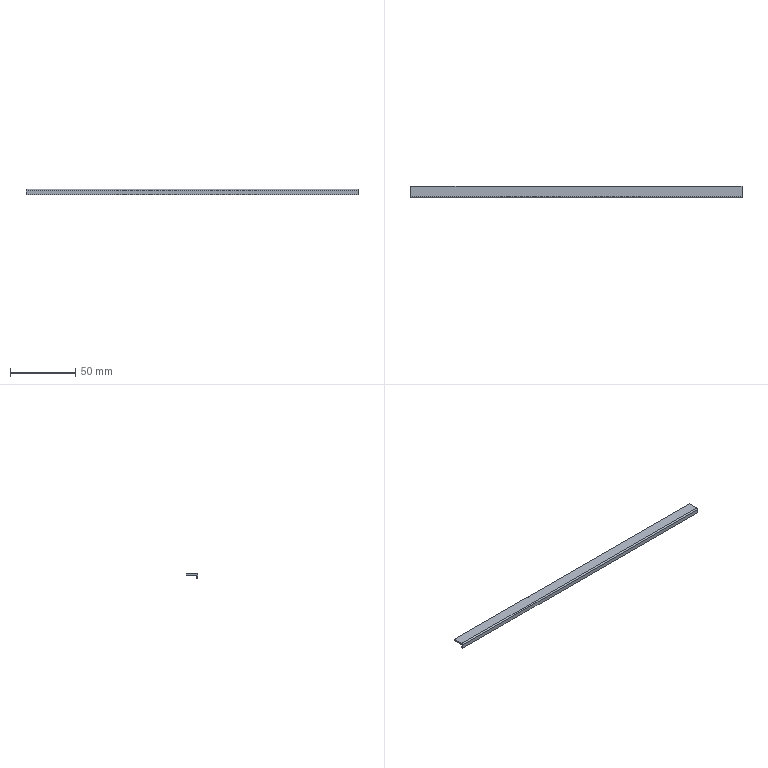Part | STEP file | gslz 2016.10.28-13_id966_x_t | 1 solid | 12 faces | box 255.209 x 9 x 4 mm | volume 3693 mm3 | plane 9 | cylinder 3 | commonest cylinder face diameters 4 x2 2 x1
STEP:
#1=CARTESIAN_POINT('',(0.,0.,0.));
#2=DIRECTION('',(0.,0.,1.));
#3=DIRECTION('',(1.,0.,0.));
#4=AXIS2_PLACEMENT_3D('',#1,#2,#3);
#5=CARTESIAN_POINT('',(-377.345,-257.,0.));
#6=VERTEX_POINT('',#5);
#7=CARTESIAN_POINT('',(-551.382,-257.,0.));
#8=VERTEX_POINT('',#7);
#9=CARTESIAN_POINT('',(-428.432,-257.,0.));
#10=DIRECTION('',(-1.,0.,0.));
#11=VECTOR('',#10,1.);
#12=LINE('',#9,#11);
#13=CARTESIAN_POINT('',(-428.432,-257.,2.5));
#14=DIRECTION('',(0.,-1.,0.));
#15=DIRECTION('',(1.,0.,0.));
#16=AXIS2_PLACEMENT_3D('',#13,#14,#15);
#17=PLANE('',#16);
#18=CARTESIAN_POINT('',(0.,-2.5));
#19=DIRECTION('',(-1.,0.));
#20=VECTOR('',#19,1.);
#21=LINE('',#18,#20);
#22=(GEOMETRIC_REPRESENTATION_CONTEXT(2)PARAMETRIC_REPRESENTATION_CONTEXT()REPRESENTATION_CONTEXT('',''));
#23=DEFINITIONAL_REPRESENTATION('',(#21),#22);
#24=PCURVE('',#17,#23);
#25=CARTESIAN_POINT('',(1793.591,319.067,0.));
#26=DIRECTION('',(0.,0.,1.));
#27=DIRECTION('',(1.,0.,0.));
#28=AXIS2_PLACEMENT_3D('',#25,#26,#27);
#29=PLANE('',#28);
#30=CARTESIAN_POINT('',(-2222.023,-576.067));
#31=DIRECTION('',(-1.,0.));
#32=VECTOR('',#31,1.);
#33=LINE('',#30,#32);
#34=(GEOMETRIC_REPRESENTATION_CONTEXT(2)PARAMETRIC_REPRESENTATION_CONTEXT()REPRESENTATION_CONTEXT('',''));
#35=DEFINITIONAL_REPRESENTATION('',(#33),#34);
#36=PCURVE('',#29,#35);
#37=SURFACE_CURVE('',#12,(#24,#36),.PCURVE_S1.);
#38=EDGE_CURVE('',#6,#8,#37,.T.);
#39=ORIENTED_EDGE('',*,*,#38,.T.);
#40=CARTESIAN_POINT('',(-551.382,-257.,1.25));
#41=VERTEX_POINT('',#40);
#42=CARTESIAN_POINT('',(-551.382,-257.,2.5));
#43=DIRECTION('',(0.,0.,-1.));
#44=VECTOR('',#43,1.);
#45=LINE('',#42,#44);
#46=CARTESIAN_POINT('',(-122.95,0.));
#47=DIRECTION('',(0.,-1.));
#48=VECTOR('',#47,1.);
#49=LINE('',#46,#48);
#50=(GEOMETRIC_REPRESENTATION_CONTEXT(2)PARAMETRIC_REPRESENTATION_CONTEXT()REPRESENTATION_CONTEXT('',''));
#51=DEFINITIONAL_REPRESENTATION('',(#49),#50);
#52=PCURVE('',#17,#51);
#53=CARTESIAN_POINT('',(-552.435,-255.3,2.5));
#54=DIRECTION('',(0.,0.,-1.));
#55=DIRECTION('',(-1.,0.,0.));
#56=AXIS2_PLACEMENT_3D('',#53,#54,#55);
#57=CYLINDRICAL_SURFACE('',#56,2.);
#58=CARTESIAN_POINT('',(4.158,0.));
#59=DIRECTION('',(0.,1.));
#60=VECTOR('',#59,1.);
#61=LINE('',#58,#60);
#62=(GEOMETRIC_REPRESENTATION_CONTEXT(2)PARAMETRIC_REPRESENTATION_CONTEXT()REPRESENTATION_CONTEXT('',''));
#63=DEFINITIONAL_REPRESENTATION('',(#61),#62);
#64=PCURVE('',#57,#63);
#65=SURFACE_CURVE('',#45,(#52,#64),.PCURVE_S1.);
#66=EDGE_CURVE('',#41,#8,#65,.T.);
#67=ORIENTED_EDGE('',*,*,#66,.F.);
#68=CARTESIAN_POINT('',(-377.345,-257.,1.25));
#69=VERTEX_POINT('',#68);
#70=CARTESIAN_POINT('',(1793.591,-257.,1.25));
#71=DIRECTION('',(1.,0.,0.));
#72=VECTOR('',#71,1.);
#73=LINE('',#70,#72);
#74=CARTESIAN_POINT('',(2222.023,-1.25));
#75=DIRECTION('',(1.,0.));
#76=VECTOR('',#75,1.);
#77=LINE('',#74,#76);
#78=(GEOMETRIC_REPRESENTATION_CONTEXT(2)PARAMETRIC_REPRESENTATION_CONTEXT()REPRESENTATION_CONTEXT('',''));
#79=DEFINITIONAL_REPRESENTATION('',(#77),#78);
#80=PCURVE('',#17,#79);
#81=CARTESIAN_POINT('',(1793.591,319.067,1.25));
#82=DIRECTION('',(0.,0.,1.));
#83=DIRECTION('',(1.,0.,0.));
#84=AXIS2_PLACEMENT_3D('',#81,#82,#83);
#85=PLANE('',#84);
#86=CARTESIAN_POINT('',(0.,-576.067));
#87=DIRECTION('',(1.,0.));
#88=VECTOR('',#87,1.);
#89=LINE('',#86,#88);
#90=(GEOMETRIC_REPRESENTATION_CONTEXT(2)PARAMETRIC_REPRESENTATION_CONTEXT()REPRESENTATION_CONTEXT('',''));
#91=DEFINITIONAL_REPRESENTATION('',(#89),#90);
#92=PCURVE('',#85,#91);
#93=SURFACE_CURVE('',#73,(#80,#92),.PCURVE_S1.);
#94=EDGE_CURVE('',#41,#69,#93,.T.);
#95=ORIENTED_EDGE('',*,*,#94,.T.);
#96=CARTESIAN_POINT('',(-377.345,-257.,-0.75));
#97=DIRECTION('',(0.,0.,1.));
#98=VECTOR('',#97,1.);
#99=LINE('',#96,#98);
#100=CARTESIAN_POINT('',(51.087,-3.25));
#101=DIRECTION('',(0.,1.));
#102=VECTOR('',#101,1.);
#103=LINE('',#100,#102);
#104=(GEOMETRIC_REPRESENTATION_CONTEXT(2)PARAMETRIC_REPRESENTATION_CONTEXT()REPRESENTATION_CONTEXT('',''));
#105=DEFINITIONAL_REPRESENTATION('',(#103),#104);
#106=PCURVE('',#17,#105);
#107=CARTESIAN_POINT('',(-377.345,-275.25,-0.75));
#108=DIRECTION('',(-1.,0.,0.));
#109=DIRECTION('',(0.,-1.,0.));
#110=AXIS2_PLACEMENT_3D('',#107,#108,#109);
#111=PLANE('',#110);
#112=CARTESIAN_POINT('',(-18.25,0.));
#113=DIRECTION('',(0.,1.));
#114=VECTOR('',#113,1.);
#115=LINE('',#112,#114);
#116=(GEOMETRIC_REPRESENTATION_CONTEXT(2)PARAMETRIC_REPRESENTATION_CONTEXT()REPRESENTATION_CONTEXT('',''));
#117=DEFINITIONAL_REPRESENTATION('',(#115),#116);
#118=PCURVE('',#111,#117);
#119=SURFACE_CURVE('',#99,(#106,#118),.PCURVE_S1.);
#120=EDGE_CURVE('',#6,#69,#119,.T.);
#121=ORIENTED_EDGE('',*,*,#120,.F.);
#122=EDGE_LOOP('',(#39,#67,#95,#121));
#123=FACE_BOUND('',#122,.T.);
#124=ADVANCED_FACE('',(#123),#17,.F.);
#125=CARTESIAN_POINT('',(-553.195,-257.15,1.25));
#126=VERTEX_POINT('',#125);
#127=CARTESIAN_POINT('',(-552.435,-255.3,1.25));
#128=DIRECTION('',(0.,0.,-1.));
#129=DIRECTION('',(1.,0.,0.));
#130=AXIS2_PLACEMENT_3D('',#127,#128,#129);
#131=CIRCLE('',#130,2.);
#132=CARTESIAN_POINT('',(3.142,1.25));
#133=DIRECTION('',(1.,0.));
#134=VECTOR('',#133,1.);
#135=LINE('',#132,#134);
#136=(GEOMETRIC_REPRESENTATION_CONTEXT(2)PARAMETRIC_REPRESENTATION_CONTEXT()REPRESENTATION_CONTEXT('',''));
#137=DEFINITIONAL_REPRESENTATION('',(#135),#136);
#138=PCURVE('',#57,#137);
#139=CARTESIAN_POINT('',(-2344.027,-574.367));
#140=CARTESIAN_POINT('',(-2344.027,-577.831));
#141=CARTESIAN_POINT('',(-2347.027,-576.099));
#142=CARTESIAN_POINT('',(-2350.027,-574.367));
#143=CARTESIAN_POINT('',(-2347.027,-572.635));
#144=CARTESIAN_POINT('',(-2344.027,-570.903));
#145=CARTESIAN_POINT('',(-2344.027,-574.367));
#146=(BOUNDED_CURVE()B_SPLINE_CURVE(2,(#139,#140,#141,#142,#143,#144,#145),.UNSPECIFIED.,.T.,.F.)B_SPLINE_CURVE_WITH_KNOTS((1,2,2,2,2,1),(-2.094,0.,2.094,4.189,6.283,8.378),.UNSPECIFIED.)CURVE()GEOMETRIC_REPRESENTATION_ITEM()RATIONAL_B_SPLINE_CURVE((1.,0.5,1.,0.5,1.,0.5,1.))REPRESENTATION_ITEM(''));
#147=(GEOMETRIC_REPRESENTATION_CONTEXT(2)PARAMETRIC_REPRESENTATION_CONTEXT()REPRESENTATION_CONTEXT('',''));
#148=DEFINITIONAL_REPRESENTATION('',(#146),#147);
#149=PCURVE('',#85,#148);
#150=SURFACE_CURVE('',#131,(#138,#149),.PCURVE_S1.);
#151=EDGE_CURVE('',#41,#126,#150,.T.);
#152=ORIENTED_EDGE('',*,*,#151,.T.);
#153=CARTESIAN_POINT('',(-553.195,-257.15,0.));
#154=VERTEX_POINT('',#153);
#155=CARTESIAN_POINT('',(-553.195,-257.15,2.5));
#156=DIRECTION('',(0.,0.,1.));
#157=VECTOR('',#156,1.);
#158=LINE('',#155,#157);
#159=CARTESIAN_POINT('',(5.102,0.));
#160=DIRECTION('',(0.,-1.));
#161=VECTOR('',#160,1.);
#162=LINE('',#159,#161);
#163=(GEOMETRIC_REPRESENTATION_CONTEXT(2)PARAMETRIC_REPRESENTATION_CONTEXT()REPRESENTATION_CONTEXT('',''));
#164=DEFINITIONAL_REPRESENTATION('',(#162),#163);
#165=PCURVE('',#57,#164);
#166=CARTESIAN_POINT('',(-553.955,-259.,2.5));
#167=DIRECTION('',(0.,0.,-1.));
#168=DIRECTION('',(-1.,0.,0.));
#169=AXIS2_PLACEMENT_3D('',#166,#167,#168);
#170=CYLINDRICAL_SURFACE('',#169,2.);
#171=CARTESIAN_POINT('',(1.961,0.));
#172=DIRECTION('',(0.,-1.));
#173=VECTOR('',#172,1.);
#174=LINE('',#171,#173);
#175=(GEOMETRIC_REPRESENTATION_CONTEXT(2)PARAMETRIC_REPRESENTATION_CONTEXT()REPRESENTATION_CONTEXT('',''));
#176=DEFINITIONAL_REPRESENTATION('',(#174),#175);
#177=PCURVE('',#170,#176);
#178=SURFACE_CURVE('',#158,(#165,#177),.PCURVE_S1.);
#179=EDGE_CURVE('',#154,#126,#178,.T.);
#180=ORIENTED_EDGE('',*,*,#179,.F.);
#181=CARTESIAN_POINT('',(-552.435,-255.3,0.));
#182=DIRECTION('',(0.,0.,1.));
#183=DIRECTION('',(1.,0.,0.));
#184=AXIS2_PLACEMENT_3D('',#181,#182,#183);
#185=CIRCLE('',#184,2.);
#186=CARTESIAN_POINT('',(9.425,2.5));
#187=DIRECTION('',(-1.,0.));
#188=VECTOR('',#187,1.);
#189=LINE('',#186,#188);
#190=(GEOMETRIC_REPRESENTATION_CONTEXT(2)PARAMETRIC_REPRESENTATION_CONTEXT()REPRESENTATION_CONTEXT('',''));
#191=DEFINITIONAL_REPRESENTATION('',(#189),#190);
#192=PCURVE('',#57,#191);
#193=CARTESIAN_POINT('',(-2346.027,-574.367));
#194=DIRECTION('',(1.,0.));
#195=AXIS2_PLACEMENT_2D('',#193,#194);
#196=CIRCLE('',#195,2.);
#197=(GEOMETRIC_REPRESENTATION_CONTEXT(2)PARAMETRIC_REPRESENTATION_CONTEXT()REPRESENTATION_CONTEXT('',''));
#198=DEFINITIONAL_REPRESENTATION('',(#196),#197);
#199=PCURVE('',#29,#198);
#200=SURFACE_CURVE('',#185,(#192,#199),.PCURVE_S1.);
#201=EDGE_CURVE('',#154,#8,#200,.T.);
#202=ORIENTED_EDGE('',*,*,#201,.T.);
#203=ORIENTED_EDGE('',*,*,#66,.F.);
#204=EDGE_LOOP('',(#152,#180,#202,#203));
#205=FACE_BOUND('',#204,.F.);
#206=ADVANCED_FACE('',(#205),#57,.F.);
#207=ORIENTED_EDGE('',*,*,#179,.F.);
#208=CARTESIAN_POINT('',(-553.955,-257.,0.));
#209=VERTEX_POINT('',#208);
#210=CARTESIAN_POINT('',(-553.955,-259.,0.));
#211=DIRECTION('',(0.,0.,-1.));
#212=DIRECTION('',(1.,0.,0.));
#213=AXIS2_PLACEMENT_3D('',#210,#211,#212);
#214=CIRCLE('',#213,2.);
#215=CARTESIAN_POINT('',(-3.142,2.5));
#216=DIRECTION('',(1.,0.));
#217=VECTOR('',#216,1.);
#218=LINE('',#215,#217);
#219=(GEOMETRIC_REPRESENTATION_CONTEXT(2)PARAMETRIC_REPRESENTATION_CONTEXT()REPRESENTATION_CONTEXT('',''));
#220=DEFINITIONAL_REPRESENTATION('',(#218),#219);
#221=PCURVE('',#170,#220);
#222=CARTESIAN_POINT('',(-2345.546,-578.067));
#223=CARTESIAN_POINT('',(-2345.546,-581.531));
#224=CARTESIAN_POINT('',(-2348.546,-579.799));
#225=CARTESIAN_POINT('',(-2351.546,-578.067));
#226=CARTESIAN_POINT('',(-2348.546,-576.335));
#227=CARTESIAN_POINT('',(-2345.546,-574.603));
#228=CARTESIAN_POINT('',(-2345.546,-578.067));
#229=(BOUNDED_CURVE()B_SPLINE_CURVE(2,(#222,#223,#224,#225,#226,#227,#228),.UNSPECIFIED.,.T.,.F.)B_SPLINE_CURVE_WITH_KNOTS((1,2,2,2,2,1),(-2.094,0.,2.094,4.189,6.283,8.378),.UNSPECIFIED.)CURVE()GEOMETRIC_REPRESENTATION_ITEM()RATIONAL_B_SPLINE_CURVE((1.,0.5,1.,0.5,1.,0.5,1.))REPRESENTATION_ITEM(''));
#230=(GEOMETRIC_REPRESENTATION_CONTEXT(2)PARAMETRIC_REPRESENTATION_CONTEXT()REPRESENTATION_CONTEXT('',''));
#231=DEFINITIONAL_REPRESENTATION('',(#229),#230);
#232=PCURVE('',#29,#231);
#233=SURFACE_CURVE('',#214,(#221,#232),.PCURVE_S1.);
#234=EDGE_CURVE('',#209,#154,#233,.T.);
#235=ORIENTED_EDGE('',*,*,#234,.F.);
#236=CARTESIAN_POINT('',(-553.955,-257.,1.25));
#237=VERTEX_POINT('',#236);
#238=CARTESIAN_POINT('',(-553.955,-257.,2.5));
#239=DIRECTION('',(0.,0.,1.));
#240=VECTOR('',#239,1.);
#241=LINE('',#238,#240);
#242=CARTESIAN_POINT('',(1.571,0.));
#243=DIRECTION('',(0.,-1.));
#244=VECTOR('',#243,1.);
#245=LINE('',#242,#244);
#246=(GEOMETRIC_REPRESENTATION_CONTEXT(2)PARAMETRIC_REPRESENTATION_CONTEXT()REPRESENTATION_CONTEXT('',''));
#247=DEFINITIONAL_REPRESENTATION('',(#245),#246);
#248=PCURVE('',#170,#247);
#249=CARTESIAN_POINT('',(-614.757,-257.,2.5));
#250=DIRECTION('',(0.,1.,0.));
#251=DIRECTION('',(-1.,0.,0.));
#252=AXIS2_PLACEMENT_3D('',#249,#250,#251);
#253=PLANE('',#252);
#254=CARTESIAN_POINT('',(-60.802,0.));
#255=DIRECTION('',(0.,1.));
#256=VECTOR('',#255,1.);
#257=LINE('',#254,#256);
#258=(GEOMETRIC_REPRESENTATION_CONTEXT(2)PARAMETRIC_REPRESENTATION_CONTEXT()REPRESENTATION_CONTEXT('',''));
#259=DEFINITIONAL_REPRESENTATION('',(#257),#258);
#260=PCURVE('',#253,#259);
#261=SURFACE_CURVE('',#241,(#248,#260),.PCURVE_S1.);
#262=EDGE_CURVE('',#209,#237,#261,.T.);
#263=ORIENTED_EDGE('',*,*,#262,.T.);
#264=CARTESIAN_POINT('',(-553.955,-259.,1.25));
#265=DIRECTION('',(0.,0.,1.));
#266=DIRECTION('',(1.,0.,0.));
#267=AXIS2_PLACEMENT_3D('',#264,#265,#266);
#268=CIRCLE('',#267,2.);
#269=CARTESIAN_POINT('',(3.142,1.25));
#270=DIRECTION('',(-1.,0.));
#271=VECTOR('',#270,1.);
#272=LINE('',#269,#271);
#273=(GEOMETRIC_REPRESENTATION_CONTEXT(2)PARAMETRIC_REPRESENTATION_CONTEXT()REPRESENTATION_CONTEXT('',''));
#274=DEFINITIONAL_REPRESENTATION('',(#272),#273);
#275=PCURVE('',#170,#274);
#276=CARTESIAN_POINT('',(-2347.546,-578.067));
#277=DIRECTION('',(1.,0.));
#278=AXIS2_PLACEMENT_2D('',#276,#277);
#279=CIRCLE('',#278,2.);
#280=(GEOMETRIC_REPRESENTATION_CONTEXT(2)PARAMETRIC_REPRESENTATION_CONTEXT()REPRESENTATION_CONTEXT('',''));
#281=DEFINITIONAL_REPRESENTATION('',(#279),#280);
#282=PCURVE('',#85,#281);
#283=SURFACE_CURVE('',#268,(#275,#282),.PCURVE_S1.);
#284=EDGE_CURVE('',#126,#237,#283,.T.);
#285=ORIENTED_EDGE('',*,*,#284,.F.);
#286=EDGE_LOOP('',(#207,#235,#263,#285));
#287=FACE_BOUND('',#286,.T.);
#288=ADVANCED_FACE('',(#287),#170,.T.);
#289=CARTESIAN_POINT('',(-377.345,-265.,1.25));
#290=VERTEX_POINT('',#289);
#291=CARTESIAN_POINT('',(-377.345,319.067,1.25));
#292=DIRECTION('',(0.,-1.,0.));
#293=VECTOR('',#292,1.);
#294=LINE('',#291,#293);
#295=CARTESIAN_POINT('',(-594.317,2.));
#296=DIRECTION('',(1.,0.));
#297=VECTOR('',#296,1.);
#298=LINE('',#295,#297);
#299=(GEOMETRIC_REPRESENTATION_CONTEXT(2)PARAMETRIC_REPRESENTATION_CONTEXT()REPRESENTATION_CONTEXT('',''));
#300=DEFINITIONAL_REPRESENTATION('',(#298),#299);
#301=PCURVE('',#111,#300);
#302=CARTESIAN_POINT('',(-2170.936,0.));
#303=DIRECTION('',(0.,-1.));
#304=VECTOR('',#303,1.);
#305=LINE('',#302,#304);
#306=(GEOMETRIC_REPRESENTATION_CONTEXT(2)PARAMETRIC_REPRESENTATION_CONTEXT()REPRESENTATION_CONTEXT('',''));
#307=DEFINITIONAL_REPRESENTATION('',(#305),#306);
#308=PCURVE('',#85,#307);
#309=SURFACE_CURVE('',#294,(#301,#308),.PCURVE_S1.);
#310=EDGE_CURVE('',#69,#290,#309,.T.);
#311=ORIENTED_EDGE('',*,*,#310,.T.);
#312=CARTESIAN_POINT('',(-377.345,-266.,0.25));
#313=VERTEX_POINT('',#312);
#314=CARTESIAN_POINT('',(-377.345,-265.,0.25));
#315=DIRECTION('',(1.,0.,0.));
#316=DIRECTION('',(0.,-1.,0.));
#317=AXIS2_PLACEMENT_3D('',#314,#315,#316);
#318=CIRCLE('',#317,1.);
#319=CARTESIAN_POINT('',(-9.25,1.));
#320=CARTESIAN_POINT('',(-9.25,-0.7321));
#321=CARTESIAN_POINT('',(-10.75,0.134));
#322=CARTESIAN_POINT('',(-12.25,1.));
#323=CARTESIAN_POINT('',(-10.75,1.866));
#324=CARTESIAN_POINT('',(-9.25,2.732));
#325=CARTESIAN_POINT('',(-9.25,1.));
#326=(BOUNDED_CURVE()B_SPLINE_CURVE(2,(#319,#320,#321,#322,#323,#324,#325),.UNSPECIFIED.,.T.,.F.)B_SPLINE_CURVE_WITH_KNOTS((1,2,2,2,2,1),(-2.094,0.,2.094,4.189,6.283,8.378),.UNSPECIFIED.)CURVE()GEOMETRIC_REPRESENTATION_ITEM()RATIONAL_B_SPLINE_CURVE((1.,0.5,1.,0.5,1.,0.5,1.))REPRESENTATION_ITEM(''));
#327=(GEOMETRIC_REPRESENTATION_CONTEXT(2)PARAMETRIC_REPRESENTATION_CONTEXT()REPRESENTATION_CONTEXT('',''));
#328=DEFINITIONAL_REPRESENTATION('',(#326),#327);
#329=PCURVE('',#111,#328);
#330=CARTESIAN_POINT('',(1793.591,-265.,0.25));
#331=DIRECTION('',(1.,0.,0.));
#332=DIRECTION('',(0.,1.,0.));
#333=AXIS2_PLACEMENT_3D('',#330,#331,#332);
#334=CYLINDRICAL_SURFACE('',#333,1.);
#335=CARTESIAN_POINT('',(-3.142,-2170.936));
#336=DIRECTION('',(1.,0.));
#337=VECTOR('',#336,1.);
#338=LINE('',#335,#337);
#339=(GEOMETRIC_REPRESENTATION_CONTEXT(2)PARAMETRIC_REPRESENTATION_CONTEXT()REPRESENTATION_CONTEXT('',''));
#340=DEFINITIONAL_REPRESENTATION('',(#338),#339);
#341=PCURVE('',#334,#340);
#342=SURFACE_CURVE('',#318,(#329,#341),.PCURVE_S1.);
#343=EDGE_CURVE('',#290,#313,#342,.T.);
#344=ORIENTED_EDGE('',*,*,#343,.T.);
#345=CARTESIAN_POINT('',(-377.345,-266.,-2.75));
#346=VERTEX_POINT('',#345);
#347=CARTESIAN_POINT('',(-377.345,-266.,-0.75));
#348=DIRECTION('',(0.,0.,1.));
#349=VECTOR('',#348,1.);
#350=LINE('',#347,#349);
#351=CARTESIAN_POINT('',(-9.25,0.));
#352=DIRECTION('',(0.,1.));
#353=VECTOR('',#352,1.);
#354=LINE('',#351,#353);
#355=(GEOMETRIC_REPRESENTATION_CONTEXT(2)PARAMETRIC_REPRESENTATION_CONTEXT()REPRESENTATION_CONTEXT('',''));
#356=DEFINITIONAL_REPRESENTATION('',(#354),#355);
#357=PCURVE('',#111,#356);
#358=CARTESIAN_POINT('',(-548.575,-266.,0.625));
#359=DIRECTION('',(0.,-1.,0.));
#360=DIRECTION('',(1.,0.,0.));
#361=AXIS2_PLACEMENT_3D('',#358,#359,#360);
#362=PLANE('',#361);
#363=CARTESIAN_POINT('',(171.229,-1.375));
#364=DIRECTION('',(0.,1.));
#365=VECTOR('',#364,1.);
#366=LINE('',#363,#365);
#367=(GEOMETRIC_REPRESENTATION_CONTEXT(2)PARAMETRIC_REPRESENTATION_CONTEXT()REPRESENTATION_CONTEXT('',''));
#368=DEFINITIONAL_REPRESENTATION('',(#366),#367);
#369=PCURVE('',#362,#368);
#370=SURFACE_CURVE('',#350,(#357,#369),.PCURVE_S1.);
#371=EDGE_CURVE('',#346,#313,#370,.T.);
#372=ORIENTED_EDGE('',*,*,#371,.F.);
#373=CARTESIAN_POINT('',(-377.345,-264.75,-2.75));
#374=VERTEX_POINT('',#373);
#375=CARTESIAN_POINT('',(-377.345,-266.,-2.75));
#376=DIRECTION('',(0.,-1.,0.));
#377=VECTOR('',#376,1.);
#378=LINE('',#375,#377);
#379=CARTESIAN_POINT('',(-9.25,-2.));
#380=DIRECTION('',(1.,0.));
#381=VECTOR('',#380,1.);
#382=LINE('',#379,#381);
#383=(GEOMETRIC_REPRESENTATION_CONTEXT(2)PARAMETRIC_REPRESENTATION_CONTEXT()REPRESENTATION_CONTEXT('',''));
#384=DEFINITIONAL_REPRESENTATION('',(#382),#383);
#385=PCURVE('',#111,#384);
#386=CARTESIAN_POINT('',(-1810.,-266.,-2.75));
#387=DIRECTION('',(0.,0.,1.));
#388=DIRECTION('',(-1.,0.,0.));
#389=AXIS2_PLACEMENT_3D('',#386,#387,#388);
#390=PLANE('',#389);
#391=CARTESIAN_POINT('',(-1432.655,0.));
#392=DIRECTION('',(0.,1.));
#393=VECTOR('',#392,1.);
#394=LINE('',#391,#393);
#395=(GEOMETRIC_REPRESENTATION_CONTEXT(2)PARAMETRIC_REPRESENTATION_CONTEXT()REPRESENTATION_CONTEXT('',''));
#396=DEFINITIONAL_REPRESENTATION('',(#394),#395);
#397=PCURVE('',#390,#396);
#398=SURFACE_CURVE('',#378,(#385,#397),.PCURVE_S1.);
#399=EDGE_CURVE('',#374,#346,#398,.T.);
#400=ORIENTED_EDGE('',*,*,#399,.F.);
#401=CARTESIAN_POINT('',(-377.345,-264.75,0.));
#402=VERTEX_POINT('',#401);
#403=CARTESIAN_POINT('',(-377.345,-264.75,-0.75));
#404=DIRECTION('',(0.,0.,1.));
#405=VECTOR('',#404,1.);
#406=LINE('',#403,#405);
#407=CARTESIAN_POINT('',(-10.5,0.));
#408=DIRECTION('',(0.,1.));
#409=VECTOR('',#408,1.);
#410=LINE('',#407,#409);
#411=(GEOMETRIC_REPRESENTATION_CONTEXT(2)PARAMETRIC_REPRESENTATION_CONTEXT()REPRESENTATION_CONTEXT('',''));
#412=DEFINITIONAL_REPRESENTATION('',(#410),#411);
#413=PCURVE('',#111,#412);
#414=CARTESIAN_POINT('',(1463.925,-264.75,-135.834));
#415=DIRECTION('',(0.,-1.,0.));
#416=DIRECTION('',(1.,0.,0.));
#417=AXIS2_PLACEMENT_3D('',#414,#415,#416);
#418=PLANE('',#417);
#419=CARTESIAN_POINT('',(-1841.271,135.084));
#420=DIRECTION('',(0.,1.));
#421=VECTOR('',#420,1.);
#422=LINE('',#419,#421);
#423=(GEOMETRIC_REPRESENTATION_CONTEXT(2)PARAMETRIC_REPRESENTATION_CONTEXT()REPRESENTATION_CONTEXT('',''));
#424=DEFINITIONAL_REPRESENTATION('',(#422),#423);
#425=PCURVE('',#418,#424);
#426=SURFACE_CURVE('',#406,(#413,#425),.PCURVE_S1.);
#427=EDGE_CURVE('',#374,#402,#426,.T.);
#428=ORIENTED_EDGE('',*,*,#427,.T.);
#429=CARTESIAN_POINT('',(-377.345,-275.25,0.));
#430=DIRECTION('',(0.,1.,0.));
#431=VECTOR('',#430,1.);
#432=LINE('',#429,#431);
#433=CARTESIAN_POINT('',(0.,0.75));
#434=DIRECTION('',(-1.,0.));
#435=VECTOR('',#434,1.);
#436=LINE('',#433,#435);
#437=(GEOMETRIC_REPRESENTATION_CONTEXT(2)PARAMETRIC_REPRESENTATION_CONTEXT()REPRESENTATION_CONTEXT('',''));
#438=DEFINITIONAL_REPRESENTATION('',(#436),#437);
#439=PCURVE('',#111,#438);
#440=CARTESIAN_POINT('',(-2170.936,-594.317));
#441=DIRECTION('',(0.,1.));
#442=VECTOR('',#441,1.);
#443=LINE('',#440,#442);
#444=(GEOMETRIC_REPRESENTATION_CONTEXT(2)PARAMETRIC_REPRESENTATION_CONTEXT()REPRESENTATION_CONTEXT('',''));
#445=DEFINITIONAL_REPRESENTATION('',(#443),#444);
#446=PCURVE('',#29,#445);
#447=SURFACE_CURVE('',#432,(#439,#446),.PCURVE_S1.);
#448=EDGE_CURVE('',#402,#6,#447,.T.);
#449=ORIENTED_EDGE('',*,*,#448,.T.);
#450=ORIENTED_EDGE('',*,*,#120,.T.);
#451=EDGE_LOOP('',(#311,#344,#372,#400,#428,#449,#450));
#452=FACE_BOUND('',#451,.T.);
#453=ADVANCED_FACE('',(#452),#111,.F.);
#454=CARTESIAN_POINT('',(-632.554,-265.,1.25));
#455=VERTEX_POINT('',#454);
#456=CARTESIAN_POINT('',(-632.554,-266.,0.25));
#457=VERTEX_POINT('',#456);
#458=CARTESIAN_POINT('',(-632.554,-265.,0.25));
#459=DIRECTION('',(1.,0.,0.));
#460=DIRECTION('',(0.,0.,-1.));
#461=AXIS2_PLACEMENT_3D('',#458,#459,#460);
#462=CIRCLE('',#461,1.);
#463=CARTESIAN_POINT('',(-1.571,-2426.145));
#464=DIRECTION('',(1.,0.));
#465=VECTOR('',#464,1.);
#466=LINE('',#463,#465);
#467=(GEOMETRIC_REPRESENTATION_CONTEXT(2)PARAMETRIC_REPRESENTATION_CONTEXT()REPRESENTATION_CONTEXT('',''));
#468=DEFINITIONAL_REPRESENTATION('',(#466),#467);
#469=PCURVE('',#334,#468);
#470=CARTESIAN_POINT('',(-632.554,-244.358,-2.25));
#471=DIRECTION('',(1.,0.,0.));
#472=DIRECTION('',(0.,0.,-1.));
#473=AXIS2_PLACEMENT_3D('',#470,#471,#472);
#474=PLANE('',#473);
#475=CARTESIAN_POINT('',(-2.5,-20.642));
#476=DIRECTION('',(1.,0.));
#477=AXIS2_PLACEMENT_2D('',#475,#476);
#478=CIRCLE('',#477,1.);
#479=(GEOMETRIC_REPRESENTATION_CONTEXT(2)PARAMETRIC_REPRESENTATION_CONTEXT()REPRESENTATION_CONTEXT('',''));
#480=DEFINITIONAL_REPRESENTATION('',(#478),#479);
#481=PCURVE('',#474,#480);
#482=SURFACE_CURVE('',#462,(#469,#481),.PCURVE_S1.);
#483=EDGE_CURVE('',#455,#457,#482,.T.);
#484=ORIENTED_EDGE('',*,*,#483,.T.);
#485=CARTESIAN_POINT('',(-548.575,-266.,0.25));
#486=DIRECTION('',(-1.,0.,0.));
#487=VECTOR('',#486,1.);
#488=LINE('',#485,#487);
#489=CARTESIAN_POINT('',(3.142,-2342.166));
#490=DIRECTION('',(0.,-1.));
#491=VECTOR('',#490,1.);
#492=LINE('',#489,#491);
#493=(GEOMETRIC_REPRESENTATION_CONTEXT(2)PARAMETRIC_REPRESENTATION_CONTEXT()REPRESENTATION_CONTEXT('',''));
#494=DEFINITIONAL_REPRESENTATION('',(#492),#493);
#495=PCURVE('',#334,#494);
#496=CARTESIAN_POINT('',(0.,-0.375));
#497=DIRECTION('',(-1.,0.));
#498=VECTOR('',#497,1.);
#499=LINE('',#496,#498);
#500=(GEOMETRIC_REPRESENTATION_CONTEXT(2)PARAMETRIC_REPRESENTATION_CONTEXT()REPRESENTATION_CONTEXT('',''));
#501=DEFINITIONAL_REPRESENTATION('',(#499),#500);
#502=PCURVE('',#362,#501);
#503=SURFACE_CURVE('',#488,(#495,#502),.PCURVE_S1.);
#504=EDGE_CURVE('',#313,#457,#503,.T.);
#505=ORIENTED_EDGE('',*,*,#504,.F.);
#506=ORIENTED_EDGE('',*,*,#343,.F.);
#507=CARTESIAN_POINT('',(1793.591,-265.,1.25));
#508=DIRECTION('',(1.,0.,0.));
#509=VECTOR('',#508,1.);
#510=LINE('',#507,#509);
#511=CARTESIAN_POINT('',(1.571,0.));
#512=DIRECTION('',(0.,1.));
#513=VECTOR('',#512,1.);
#514=LINE('',#511,#513);
#515=(GEOMETRIC_REPRESENTATION_CONTEXT(2)PARAMETRIC_REPRESENTATION_CONTEXT()REPRESENTATION_CONTEXT('',''));
#516=DEFINITIONAL_REPRESENTATION('',(#514),#515);
#517=PCURVE('',#334,#516);
#518=CARTESIAN_POINT('',(0.,-584.067));
#519=DIRECTION('',(1.,0.));
#520=VECTOR('',#519,1.);
#521=LINE('',#518,#520);
#522=(GEOMETRIC_REPRESENTATION_CONTEXT(2)PARAMETRIC_REPRESENTATION_CONTEXT()REPRESENTATION_CONTEXT('',''));
#523=DEFINITIONAL_REPRESENTATION('',(#521),#522);
#524=PCURVE('',#85,#523);
#525=SURFACE_CURVE('',#510,(#517,#524),.PCURVE_S1.);
#526=EDGE_CURVE('',#455,#290,#525,.T.);
#527=ORIENTED_EDGE('',*,*,#526,.F.);
#528=EDGE_LOOP('',(#484,#505,#506,#527));
#529=FACE_BOUND('',#528,.T.);
#530=ADVANCED_FACE('',(#529),#334,.T.);
#531=CARTESIAN_POINT('',(-632.554,-266.,-2.75));
#532=VERTEX_POINT('',#531);
#533=CARTESIAN_POINT('',(-632.554,-266.,0.625));
#534=DIRECTION('',(0.,0.,1.));
#535=VECTOR('',#534,1.);
#536=LINE('',#533,#535);
#537=CARTESIAN_POINT('',(-83.979,0.));
#538=DIRECTION('',(0.,1.));
#539=VECTOR('',#538,1.);
#540=LINE('',#537,#539);
#541=(GEOMETRIC_REPRESENTATION_CONTEXT(2)PARAMETRIC_REPRESENTATION_CONTEXT()REPRESENTATION_CONTEXT('',''));
#542=DEFINITIONAL_REPRESENTATION('',(#540),#541);
#543=PCURVE('',#362,#542);
#544=CARTESIAN_POINT('',(-2.875,-21.642));
#545=DIRECTION('',(-1.,0.));
#546=VECTOR('',#545,1.);
#547=LINE('',#544,#546);
#548=(GEOMETRIC_REPRESENTATION_CONTEXT(2)PARAMETRIC_REPRESENTATION_CONTEXT()REPRESENTATION_CONTEXT('',''));
#549=DEFINITIONAL_REPRESENTATION('',(#547),#548);
#550=PCURVE('',#474,#549);
#551=SURFACE_CURVE('',#536,(#543,#550),.PCURVE_S1.);
#552=EDGE_CURVE('',#532,#457,#551,.T.);
#553=ORIENTED_EDGE('',*,*,#552,.F.);
#554=CARTESIAN_POINT('',(-1810.,-266.,-2.75));
#555=DIRECTION('',(-1.,0.,0.));
#556=VECTOR('',#555,1.);
#557=LINE('',#554,#556);
#558=CARTESIAN_POINT('',(-1261.425,-3.375));
#559=DIRECTION('',(-1.,0.));
#560=VECTOR('',#559,1.);
#561=LINE('',#558,#560);
#562=(GEOMETRIC_REPRESENTATION_CONTEXT(2)PARAMETRIC_REPRESENTATION_CONTEXT()REPRESENTATION_CONTEXT('',''));
#563=DEFINITIONAL_REPRESENTATION('',(#561),#562);
#564=PCURVE('',#362,#563);
#565=CARTESIAN_POINT('',(0.,0.));
#566=DIRECTION('',(1.,0.));
#567=VECTOR('',#566,1.);
#568=LINE('',#565,#567);
#569=(GEOMETRIC_REPRESENTATION_CONTEXT(2)PARAMETRIC_REPRESENTATION_CONTEXT()REPRESENTATION_CONTEXT('',''));
#570=DEFINITIONAL_REPRESENTATION('',(#568),#569);
#571=PCURVE('',#390,#570);
#572=SURFACE_CURVE('',#557,(#564,#571),.PCURVE_S1.);
#573=EDGE_CURVE('',#346,#532,#572,.T.);
#574=ORIENTED_EDGE('',*,*,#573,.F.);
#575=ORIENTED_EDGE('',*,*,#371,.T.);
#576=ORIENTED_EDGE('',*,*,#504,.T.);
#577=EDGE_LOOP('',(#553,#574,#575,#576));
#578=FACE_BOUND('',#577,.T.);
#579=ADVANCED_FACE('',(#578),#362,.T.);
#580=ORIENTED_EDGE('',*,*,#573,.T.);
#581=CARTESIAN_POINT('',(-632.554,-264.75,-2.75));
#582=VERTEX_POINT('',#581);
#583=CARTESIAN_POINT('',(-632.554,-266.,-2.75));
#584=DIRECTION('',(0.,-1.,0.));
#585=VECTOR('',#584,1.);
#586=LINE('',#583,#585);
#587=CARTESIAN_POINT('',(-1177.446,0.));
#588=DIRECTION('',(0.,1.));
#589=VECTOR('',#588,1.);
#590=LINE('',#587,#589);
#591=(GEOMETRIC_REPRESENTATION_CONTEXT(2)PARAMETRIC_REPRESENTATION_CONTEXT()REPRESENTATION_CONTEXT('',''));
#592=DEFINITIONAL_REPRESENTATION('',(#590),#591);
#593=PCURVE('',#390,#592);
#594=CARTESIAN_POINT('',(0.5,-21.642));
#595=DIRECTION('',(0.,-1.));
#596=VECTOR('',#595,1.);
#597=LINE('',#594,#596);
#598=(GEOMETRIC_REPRESENTATION_CONTEXT(2)PARAMETRIC_REPRESENTATION_CONTEXT()REPRESENTATION_CONTEXT('',''));
#599=DEFINITIONAL_REPRESENTATION('',(#597),#598);
#600=PCURVE('',#474,#599);
#601=SURFACE_CURVE('',#586,(#593,#600),.PCURVE_S1.);
#602=EDGE_CURVE('',#582,#532,#601,.T.);
#603=ORIENTED_EDGE('',*,*,#602,.F.);
#604=CARTESIAN_POINT('',(-1810.,-264.75,-2.75));
#605=DIRECTION('',(-1.,0.,0.));
#606=VECTOR('',#605,1.);
#607=LINE('',#604,#606);
#608=CARTESIAN_POINT('',(0.,-1.25));
#609=DIRECTION('',(1.,0.));
#610=VECTOR('',#609,1.);
#611=LINE('',#608,#610);
#612=(GEOMETRIC_REPRESENTATION_CONTEXT(2)PARAMETRIC_REPRESENTATION_CONTEXT()REPRESENTATION_CONTEXT('',''));
#613=DEFINITIONAL_REPRESENTATION('',(#611),#612);
#614=PCURVE('',#390,#613);
#615=CARTESIAN_POINT('',(-3273.925,133.084));
#616=DIRECTION('',(-1.,0.));
#617=VECTOR('',#616,1.);
#618=LINE('',#615,#617);
#619=(GEOMETRIC_REPRESENTATION_CONTEXT(2)PARAMETRIC_REPRESENTATION_CONTEXT()REPRESENTATION_CONTEXT('',''));
#620=DEFINITIONAL_REPRESENTATION('',(#618),#619);
#621=PCURVE('',#418,#620);
#622=SURFACE_CURVE('',#607,(#614,#621),.PCURVE_S1.);
#623=EDGE_CURVE('',#374,#582,#622,.T.);
#624=ORIENTED_EDGE('',*,*,#623,.F.);
#625=ORIENTED_EDGE('',*,*,#399,.T.);
#626=EDGE_LOOP('',(#580,#603,#624,#625));
#627=FACE_BOUND('',#626,.T.);
#628=ADVANCED_FACE('',(#627),#390,.F.);
#629=ORIENTED_EDGE('',*,*,#623,.T.);
#630=CARTESIAN_POINT('',(-632.554,-264.75,0.));
#631=VERTEX_POINT('',#630);
#632=CARTESIAN_POINT('',(-632.554,-264.75,-135.834));
#633=DIRECTION('',(0.,0.,1.));
#634=VECTOR('',#633,1.);
#635=LINE('',#632,#634);
#636=CARTESIAN_POINT('',(-2096.479,0.));
#637=DIRECTION('',(0.,1.));
#638=VECTOR('',#637,1.);
#639=LINE('',#636,#638);
#640=(GEOMETRIC_REPRESENTATION_CONTEXT(2)PARAMETRIC_REPRESENTATION_CONTEXT()REPRESENTATION_CONTEXT('',''));
#641=DEFINITIONAL_REPRESENTATION('',(#639),#640);
#642=PCURVE('',#418,#641);
#643=CARTESIAN_POINT('',(133.584,-20.392));
#644=DIRECTION('',(-1.,0.));
#645=VECTOR('',#644,1.);
#646=LINE('',#643,#645);
#647=(GEOMETRIC_REPRESENTATION_CONTEXT(2)PARAMETRIC_REPRESENTATION_CONTEXT()REPRESENTATION_CONTEXT('',''));
#648=DEFINITIONAL_REPRESENTATION('',(#646),#647);
#649=PCURVE('',#474,#648);
#650=SURFACE_CURVE('',#635,(#642,#649),.PCURVE_S1.);
#651=EDGE_CURVE('',#582,#631,#650,.T.);
#652=ORIENTED_EDGE('',*,*,#651,.T.);
#653=CARTESIAN_POINT('',(1793.591,-264.75,0.));
#654=DIRECTION('',(1.,0.,0.));
#655=VECTOR('',#654,1.);
#656=LINE('',#653,#655);
#657=CARTESIAN_POINT('',(329.666,135.834));
#658=DIRECTION('',(1.,0.));
#659=VECTOR('',#658,1.);
#660=LINE('',#657,#659);
#661=(GEOMETRIC_REPRESENTATION_CONTEXT(2)PARAMETRIC_REPRESENTATION_CONTEXT()REPRESENTATION_CONTEXT('',''));
#662=DEFINITIONAL_REPRESENTATION('',(#660),#661);
#663=PCURVE('',#418,#662);
#664=CARTESIAN_POINT('',(0.,-583.817));
#665=DIRECTION('',(1.,0.));
#666=VECTOR('',#665,1.);
#667=LINE('',#664,#666);
#668=(GEOMETRIC_REPRESENTATION_CONTEXT(2)PARAMETRIC_REPRESENTATION_CONTEXT()REPRESENTATION_CONTEXT('',''));
#669=DEFINITIONAL_REPRESENTATION('',(#667),#668);
#670=PCURVE('',#29,#669);
#671=SURFACE_CURVE('',#656,(#663,#670),.PCURVE_S1.);
#672=EDGE_CURVE('',#631,#402,#671,.T.);
#673=ORIENTED_EDGE('',*,*,#672,.T.);
#674=ORIENTED_EDGE('',*,*,#427,.F.);
#675=EDGE_LOOP('',(#629,#652,#673,#674));
#676=FACE_BOUND('',#675,.T.);
#677=ADVANCED_FACE('',(#676),#418,.F.);
#678=ORIENTED_EDGE('',*,*,#672,.F.);
#679=CARTESIAN_POINT('',(-632.554,-257.,0.));
#680=VERTEX_POINT('',#679);
#681=CARTESIAN_POINT('',(-632.554,319.067,0.));
#682=DIRECTION('',(0.,1.,0.));
#683=VECTOR('',#682,1.);
#684=LINE('',#681,#683);
#685=CARTESIAN_POINT('',(-2426.145,0.));
#686=DIRECTION('',(0.,1.));
#687=VECTOR('',#686,1.);
#688=LINE('',#685,#687);
#689=(GEOMETRIC_REPRESENTATION_CONTEXT(2)PARAMETRIC_REPRESENTATION_CONTEXT()REPRESENTATION_CONTEXT('',''));
#690=DEFINITIONAL_REPRESENTATION('',(#688),#689);
#691=PCURVE('',#29,#690);
#692=CARTESIAN_POINT('',(-2.25,563.425));
#693=DIRECTION('',(0.,1.));
#694=VECTOR('',#693,1.);
#695=LINE('',#692,#694);
#696=(GEOMETRIC_REPRESENTATION_CONTEXT(2)PARAMETRIC_REPRESENTATION_CONTEXT()REPRESENTATION_CONTEXT('',''));
#697=DEFINITIONAL_REPRESENTATION('',(#695),#696);
#698=PCURVE('',#474,#697);
#699=SURFACE_CURVE('',#684,(#691,#698),.PCURVE_S1.);
#700=EDGE_CURVE('',#631,#680,#699,.T.);
#701=ORIENTED_EDGE('',*,*,#700,.T.);
#702=CARTESIAN_POINT('',(-614.757,-257.,0.));
#703=DIRECTION('',(1.,0.,0.));
#704=VECTOR('',#703,1.);
#705=LINE('',#702,#704);
#706=CARTESIAN_POINT('',(-2408.349,-576.067));
#707=DIRECTION('',(1.,0.));
#708=VECTOR('',#707,1.);
#709=LINE('',#706,#708);
#710=(GEOMETRIC_REPRESENTATION_CONTEXT(2)PARAMETRIC_REPRESENTATION_CONTEXT()REPRESENTATION_CONTEXT('',''));
#711=DEFINITIONAL_REPRESENTATION('',(#709),#710);
#712=PCURVE('',#29,#711);
#713=CARTESIAN_POINT('',(0.,-2.5));
#714=DIRECTION('',(-1.,0.));
#715=VECTOR('',#714,1.);
#716=LINE('',#713,#715);
#717=(GEOMETRIC_REPRESENTATION_CONTEXT(2)PARAMETRIC_REPRESENTATION_CONTEXT()REPRESENTATION_CONTEXT('',''));
#718=DEFINITIONAL_REPRESENTATION('',(#716),#717);
#719=PCURVE('',#253,#718);
#720=SURFACE_CURVE('',#705,(#712,#719),.PCURVE_S1.);
#721=EDGE_CURVE('',#680,#209,#720,.T.);
#722=ORIENTED_EDGE('',*,*,#721,.T.);
#723=ORIENTED_EDGE('',*,*,#234,.T.);
#724=ORIENTED_EDGE('',*,*,#201,.T.);
#725=ORIENTED_EDGE('',*,*,#38,.F.);
#726=ORIENTED_EDGE('',*,*,#448,.F.);
#727=EDGE_LOOP('',(#678,#701,#722,#723,#724,#725,#726));
#728=FACE_BOUND('',#727,.T.);
#729=ADVANCED_FACE('',(#728),#29,.F.);
#730=CARTESIAN_POINT('',(-632.554,-257.,1.25));
#731=VERTEX_POINT('',#730);
#732=CARTESIAN_POINT('',(-632.554,319.067,1.25));
#733=DIRECTION('',(0.,-1.,0.));
#734=VECTOR('',#733,1.);
#735=LINE('',#732,#734);
#736=CARTESIAN_POINT('',(-2426.145,0.));
#737=DIRECTION('',(0.,-1.));
#738=VECTOR('',#737,1.);
#739=LINE('',#736,#738);
#740=(GEOMETRIC_REPRESENTATION_CONTEXT(2)PARAMETRIC_REPRESENTATION_CONTEXT()REPRESENTATION_CONTEXT('',''));
#741=DEFINITIONAL_REPRESENTATION('',(#739),#740);
#742=PCURVE('',#85,#741);
#743=CARTESIAN_POINT('',(-3.5,563.425));
#744=DIRECTION('',(0.,-1.));
#745=VECTOR('',#744,1.);
#746=LINE('',#743,#745);
#747=(GEOMETRIC_REPRESENTATION_CONTEXT(2)PARAMETRIC_REPRESENTATION_CONTEXT()REPRESENTATION_CONTEXT('',''));
#748=DEFINITIONAL_REPRESENTATION('',(#746),#747);
#749=PCURVE('',#474,#748);
#750=SURFACE_CURVE('',#735,(#742,#749),.PCURVE_S1.);
#751=EDGE_CURVE('',#731,#455,#750,.T.);
#752=ORIENTED_EDGE('',*,*,#751,.T.);
#753=ORIENTED_EDGE('',*,*,#526,.T.);
#754=ORIENTED_EDGE('',*,*,#310,.F.);
#755=ORIENTED_EDGE('',*,*,#94,.F.);
#756=ORIENTED_EDGE('',*,*,#151,.T.);
#757=ORIENTED_EDGE('',*,*,#284,.T.);
#758=CARTESIAN_POINT('',(-625.757,-257.,1.25));
#759=VERTEX_POINT('',#758);
#760=CARTESIAN_POINT('',(1793.591,-257.,1.25));
#761=DIRECTION('',(1.,0.,0.));
#762=VECTOR('',#761,1.);
#763=LINE('',#760,#762);
#764=CARTESIAN_POINT('',(0.,-576.067));
#765=DIRECTION('',(1.,0.));
#766=VECTOR('',#765,1.);
#767=LINE('',#764,#766);
#768=(GEOMETRIC_REPRESENTATION_CONTEXT(2)PARAMETRIC_REPRESENTATION_CONTEXT()REPRESENTATION_CONTEXT('',''));
#769=DEFINITIONAL_REPRESENTATION('',(#767),#768);
#770=PCURVE('',#85,#769);
#771=CARTESIAN_POINT('',(-2408.349,-1.25));
#772=DIRECTION('',(-1.,0.));
#773=VECTOR('',#772,1.);
#774=LINE('',#771,#773);
#775=(GEOMETRIC_REPRESENTATION_CONTEXT(2)PARAMETRIC_REPRESENTATION_CONTEXT()REPRESENTATION_CONTEXT('',''));
#776=DEFINITIONAL_REPRESENTATION('',(#774),#775);
#777=PCURVE('',#253,#776);
#778=SURFACE_CURVE('',#763,(#770,#777),.PCURVE_S1.);
#779=EDGE_CURVE('',#759,#237,#778,.T.);
#780=ORIENTED_EDGE('',*,*,#779,.F.);
#781=CARTESIAN_POINT('',(1793.591,-257.,1.25));
#782=DIRECTION('',(1.,0.,0.));
#783=VECTOR('',#782,1.);
#784=LINE('',#781,#783);
#785=CARTESIAN_POINT('',(-0.00000001,-576.067));
#786=DIRECTION('',(1.,0.));
#787=VECTOR('',#786,1.);
#788=LINE('',#785,#787);
#789=(GEOMETRIC_REPRESENTATION_CONTEXT(2)PARAMETRIC_REPRESENTATION_CONTEXT()REPRESENTATION_CONTEXT('',''));
#790=DEFINITIONAL_REPRESENTATION('',(#788),#789);
#791=PCURVE('',#85,#790);
#792=CARTESIAN_POINT('',(-2408.349,-1.25));
#793=DIRECTION('',(-1.,0.));
#794=VECTOR('',#793,1.);
#795=LINE('',#792,#794);
#796=(GEOMETRIC_REPRESENTATION_CONTEXT(2)PARAMETRIC_REPRESENTATION_CONTEXT()REPRESENTATION_CONTEXT('',''));
#797=DEFINITIONAL_REPRESENTATION('',(#795),#796);
#798=PCURVE('',#253,#797);
#799=SURFACE_CURVE('',#784,(#791,#798),.PCURVE_S1.);
#800=EDGE_CURVE('',#731,#759,#799,.T.);
#801=ORIENTED_EDGE('',*,*,#800,.F.);
#802=EDGE_LOOP('',(#752,#753,#754,#755,#756,#757,#780,#801));
#803=FACE_BOUND('',#802,.T.);
#804=ADVANCED_FACE('',(#803),#85,.T.);
#805=CARTESIAN_POINT('',(-632.554,-257.,2.5));
#806=DIRECTION('',(0.,0.,-1.));
#807=VECTOR('',#806,1.);
#808=LINE('',#805,#807);
#809=CARTESIAN_POINT('',(17.796,0.));
#810=DIRECTION('',(0.,-1.));
#811=VECTOR('',#810,1.);
#812=LINE('',#809,#811);
#813=(GEOMETRIC_REPRESENTATION_CONTEXT(2)PARAMETRIC_REPRESENTATION_CONTEXT()REPRESENTATION_CONTEXT('',''));
#814=DEFINITIONAL_REPRESENTATION('',(#812),#813);
#815=PCURVE('',#253,#814);
#816=CARTESIAN_POINT('',(-4.75,-12.642));
#817=DIRECTION('',(1.,0.));
#818=VECTOR('',#817,1.);
#819=LINE('',#816,#818);
#820=(GEOMETRIC_REPRESENTATION_CONTEXT(2)PARAMETRIC_REPRESENTATION_CONTEXT()REPRESENTATION_CONTEXT('',''));
#821=DEFINITIONAL_REPRESENTATION('',(#819),#820);
#822=PCURVE('',#474,#821);
#823=SURFACE_CURVE('',#808,(#815,#822),.PCURVE_S1.);
#824=EDGE_CURVE('',#731,#680,#823,.T.);
#825=ORIENTED_EDGE('',*,*,#824,.F.);
#826=ORIENTED_EDGE('',*,*,#800,.T.);
#827=ORIENTED_EDGE('',*,*,#779,.T.);
#828=ORIENTED_EDGE('',*,*,#262,.F.);
#829=ORIENTED_EDGE('',*,*,#721,.F.);
#830=EDGE_LOOP('',(#825,#826,#827,#828,#829));
#831=FACE_BOUND('',#830,.T.);
#832=ADVANCED_FACE('',(#831),#253,.T.);
#833=ORIENTED_EDGE('',*,*,#824,.T.);
#834=ORIENTED_EDGE('',*,*,#700,.F.);
#835=ORIENTED_EDGE('',*,*,#651,.F.);
#836=ORIENTED_EDGE('',*,*,#602,.T.);
#837=ORIENTED_EDGE('',*,*,#552,.T.);
#838=ORIENTED_EDGE('',*,*,#483,.F.);
#839=ORIENTED_EDGE('',*,*,#751,.F.);
#840=EDGE_LOOP('',(#833,#834,#835,#836,#837,#838,#839));
#841=FACE_BOUND('',#840,.T.);
#842=ADVANCED_FACE('',(#841),#474,.F.);
#843=CLOSED_SHELL('',(#124,#206,#288,#453,#530,#579,#628,#677,#729,#804,#832,#842));
#844=MANIFOLD_SOLID_BREP('',#843);
#845=(LENGTH_UNIT()NAMED_UNIT(*)SI_UNIT(.MILLI.,.METRE.));
#846=UNCERTAINTY_MEASURE_WITH_UNIT(LENGTH_MEASURE(0.0000001),#845,'','');
#847=(NAMED_UNIT(*)PLANE_ANGLE_UNIT()SI_UNIT($,.RADIAN.));
#848=(NAMED_UNIT(*)SI_UNIT($,.STERADIAN.)SOLID_ANGLE_UNIT());
#849=(GEOMETRIC_REPRESENTATION_CONTEXT(3)GLOBAL_UNCERTAINTY_ASSIGNED_CONTEXT((#846))GLOBAL_UNIT_ASSIGNED_CONTEXT((#845,#847,#848))REPRESENTATION_CONTEXT('',''));
#850=ADVANCED_BREP_SHAPE_REPRESENTATION('',(#4,#844),#849);